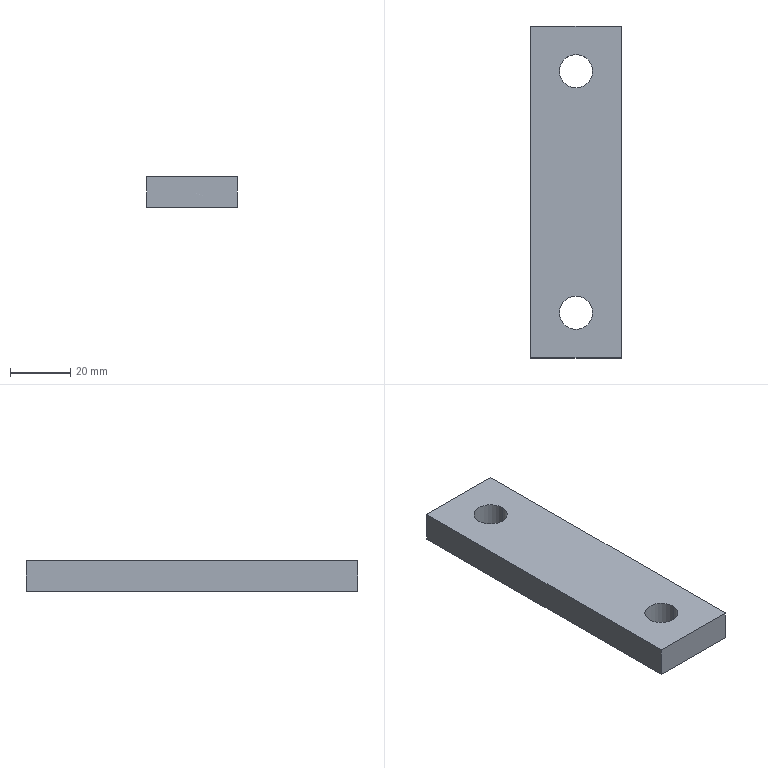Part | STEP file | Adjusting plate clamp | 1 solid | 10 faces | box 30 x 110 x 10 mm | volume 31099 mm3 | plane 6 | cylinder 4 | commonest cylinder face diameters 11 x4
STEP:
#1=CARTESIAN_POINT('',(0.,0.,0.));
#2=DIRECTION('',(0.,0.,1.));
#3=DIRECTION('',(1.,0.,0.));
#4=AXIS2_PLACEMENT_3D('',#1,#2,#3);
#5=CARTESIAN_POINT('',(5.5,-40.,-10.));
#6=VERTEX_POINT('',#5);
#7=CARTESIAN_POINT('',(5.5,-40.,0.));
#8=VERTEX_POINT('',#7);
#9=CARTESIAN_POINT('',(5.5,-40.,-10.));
#10=DIRECTION('',(0.,0.,1.));
#11=VECTOR('',#10,1.);
#12=LINE('',#9,#11);
#13=CARTESIAN_POINT('',(0.,-40.,-10.));
#14=DIRECTION('',(0.,0.,1.));
#15=DIRECTION('',(1.,0.,0.));
#16=AXIS2_PLACEMENT_3D('',#13,#14,#15);
#17=CYLINDRICAL_SURFACE('',#16,5.5);
#18=CARTESIAN_POINT('',(6.283,0.));
#19=DIRECTION('',(0.,1.));
#20=VECTOR('',#19,1.);
#21=LINE('',#18,#20);
#22=(GEOMETRIC_REPRESENTATION_CONTEXT(2)PARAMETRIC_REPRESENTATION_CONTEXT()REPRESENTATION_CONTEXT('',''));
#23=DEFINITIONAL_REPRESENTATION('',(#21),#22);
#24=PCURVE('',#17,#23);
#25=CARTESIAN_POINT('',(0.,-40.,-10.));
#26=DIRECTION('',(0.,0.,1.));
#27=DIRECTION('',(1.,0.,0.));
#28=AXIS2_PLACEMENT_3D('',#25,#26,#27);
#29=CYLINDRICAL_SURFACE('',#28,5.5);
#30=CARTESIAN_POINT('',(0.,0.));
#31=DIRECTION('',(0.,1.));
#32=VECTOR('',#31,1.);
#33=LINE('',#30,#32);
#34=(GEOMETRIC_REPRESENTATION_CONTEXT(2)PARAMETRIC_REPRESENTATION_CONTEXT()REPRESENTATION_CONTEXT('',''));
#35=DEFINITIONAL_REPRESENTATION('',(#33),#34);
#36=PCURVE('',#29,#35);
#37=SURFACE_CURVE('',#12,(#24,#36),.PCURVE_S1.);
#38=EDGE_CURVE('',#6,#8,#37,.T.);
#39=ORIENTED_EDGE('',*,*,#38,.T.);
#40=CARTESIAN_POINT('',(-5.5,-40.,0.));
#41=VERTEX_POINT('',#40);
#42=CARTESIAN_POINT('',(0.,-40.,0.));
#43=DIRECTION('',(0.,0.,1.));
#44=DIRECTION('',(1.,0.,0.));
#45=AXIS2_PLACEMENT_3D('',#42,#43,#44);
#46=CIRCLE('',#45,5.5);
#47=CARTESIAN_POINT('',(0.,10.));
#48=DIRECTION('',(1.,0.));
#49=VECTOR('',#48,1.);
#50=LINE('',#47,#49);
#51=(GEOMETRIC_REPRESENTATION_CONTEXT(2)PARAMETRIC_REPRESENTATION_CONTEXT()REPRESENTATION_CONTEXT('',''));
#52=DEFINITIONAL_REPRESENTATION('',(#50),#51);
#53=PCURVE('',#17,#52);
#54=CARTESIAN_POINT('',(0.,0.,0.));
#55=DIRECTION('',(0.,0.,1.));
#56=DIRECTION('',(1.,0.,0.));
#57=AXIS2_PLACEMENT_3D('',#54,#55,#56);
#58=PLANE('',#57);
#59=CARTESIAN_POINT('',(0.,-40.));
#60=DIRECTION('',(1.,0.));
#61=AXIS2_PLACEMENT_2D('',#59,#60);
#62=CIRCLE('',#61,5.5);
#63=(GEOMETRIC_REPRESENTATION_CONTEXT(2)PARAMETRIC_REPRESENTATION_CONTEXT()REPRESENTATION_CONTEXT('',''));
#64=DEFINITIONAL_REPRESENTATION('',(#62),#63);
#65=PCURVE('',#58,#64);
#66=SURFACE_CURVE('',#46,(#53,#65),.PCURVE_S1.);
#67=EDGE_CURVE('',#41,#8,#66,.T.);
#68=ORIENTED_EDGE('',*,*,#67,.F.);
#69=CARTESIAN_POINT('',(-5.5,-40.,-10.));
#70=VERTEX_POINT('',#69);
#71=CARTESIAN_POINT('',(-5.5,-40.,-10.));
#72=DIRECTION('',(0.,0.,1.));
#73=VECTOR('',#72,1.);
#74=LINE('',#71,#73);
#75=CARTESIAN_POINT('',(3.142,0.));
#76=DIRECTION('',(0.,1.));
#77=VECTOR('',#76,1.);
#78=LINE('',#75,#77);
#79=(GEOMETRIC_REPRESENTATION_CONTEXT(2)PARAMETRIC_REPRESENTATION_CONTEXT()REPRESENTATION_CONTEXT('',''));
#80=DEFINITIONAL_REPRESENTATION('',(#78),#79);
#81=PCURVE('',#17,#80);
#82=CARTESIAN_POINT('',(3.142,0.));
#83=DIRECTION('',(0.,1.));
#84=VECTOR('',#83,1.);
#85=LINE('',#82,#84);
#86=(GEOMETRIC_REPRESENTATION_CONTEXT(2)PARAMETRIC_REPRESENTATION_CONTEXT()REPRESENTATION_CONTEXT('',''));
#87=DEFINITIONAL_REPRESENTATION('',(#85),#86);
#88=PCURVE('',#29,#87);
#89=SURFACE_CURVE('',#74,(#81,#88),.PCURVE_S1.);
#90=EDGE_CURVE('',#70,#41,#89,.T.);
#91=ORIENTED_EDGE('',*,*,#90,.F.);
#92=CARTESIAN_POINT('',(0.,-40.,-10.));
#93=DIRECTION('',(0.,0.,1.));
#94=DIRECTION('',(1.,0.,0.));
#95=AXIS2_PLACEMENT_3D('',#92,#93,#94);
#96=CIRCLE('',#95,5.5);
#97=CARTESIAN_POINT('',(0.,0.));
#98=DIRECTION('',(1.,0.));
#99=VECTOR('',#98,1.);
#100=LINE('',#97,#99);
#101=(GEOMETRIC_REPRESENTATION_CONTEXT(2)PARAMETRIC_REPRESENTATION_CONTEXT()REPRESENTATION_CONTEXT('',''));
#102=DEFINITIONAL_REPRESENTATION('',(#100),#101);
#103=PCURVE('',#17,#102);
#104=CARTESIAN_POINT('',(0.,0.,-10.));
#105=DIRECTION('',(0.,0.,1.));
#106=DIRECTION('',(1.,0.,0.));
#107=AXIS2_PLACEMENT_3D('',#104,#105,#106);
#108=PLANE('',#107);
#109=CARTESIAN_POINT('',(0.,-40.));
#110=DIRECTION('',(1.,0.));
#111=AXIS2_PLACEMENT_2D('',#109,#110);
#112=CIRCLE('',#111,5.5);
#113=(GEOMETRIC_REPRESENTATION_CONTEXT(2)PARAMETRIC_REPRESENTATION_CONTEXT()REPRESENTATION_CONTEXT('',''));
#114=DEFINITIONAL_REPRESENTATION('',(#112),#113);
#115=PCURVE('',#108,#114);
#116=SURFACE_CURVE('',#96,(#103,#115),.PCURVE_S1.);
#117=EDGE_CURVE('',#70,#6,#116,.T.);
#118=ORIENTED_EDGE('',*,*,#117,.T.);
#119=EDGE_LOOP('',(#39,#68,#91,#118));
#120=FACE_BOUND('',#119,.F.);
#121=ADVANCED_FACE('',(#120),#17,.F.);
#122=CARTESIAN_POINT('',(5.5,40.,-10.));
#123=VERTEX_POINT('',#122);
#124=CARTESIAN_POINT('',(5.5,40.,0.));
#125=VERTEX_POINT('',#124);
#126=CARTESIAN_POINT('',(5.5,40.,-10.));
#127=DIRECTION('',(0.,0.,1.));
#128=VECTOR('',#127,1.);
#129=LINE('',#126,#128);
#130=CARTESIAN_POINT('',(0.,40.,-10.));
#131=DIRECTION('',(0.,0.,1.));
#132=DIRECTION('',(1.,0.,0.));
#133=AXIS2_PLACEMENT_3D('',#130,#131,#132);
#134=CYLINDRICAL_SURFACE('',#133,5.5);
#135=CARTESIAN_POINT('',(6.283,0.));
#136=DIRECTION('',(0.,1.));
#137=VECTOR('',#136,1.);
#138=LINE('',#135,#137);
#139=(GEOMETRIC_REPRESENTATION_CONTEXT(2)PARAMETRIC_REPRESENTATION_CONTEXT()REPRESENTATION_CONTEXT('',''));
#140=DEFINITIONAL_REPRESENTATION('',(#138),#139);
#141=PCURVE('',#134,#140);
#142=CARTESIAN_POINT('',(0.,40.,-10.));
#143=DIRECTION('',(0.,0.,1.));
#144=DIRECTION('',(1.,0.,0.));
#145=AXIS2_PLACEMENT_3D('',#142,#143,#144);
#146=CYLINDRICAL_SURFACE('',#145,5.5);
#147=CARTESIAN_POINT('',(0.,0.));
#148=DIRECTION('',(0.,1.));
#149=VECTOR('',#148,1.);
#150=LINE('',#147,#149);
#151=(GEOMETRIC_REPRESENTATION_CONTEXT(2)PARAMETRIC_REPRESENTATION_CONTEXT()REPRESENTATION_CONTEXT('',''));
#152=DEFINITIONAL_REPRESENTATION('',(#150),#151);
#153=PCURVE('',#146,#152);
#154=SURFACE_CURVE('',#129,(#141,#153),.PCURVE_S1.);
#155=EDGE_CURVE('',#123,#125,#154,.T.);
#156=ORIENTED_EDGE('',*,*,#155,.T.);
#157=CARTESIAN_POINT('',(-5.5,40.,0.));
#158=VERTEX_POINT('',#157);
#159=CARTESIAN_POINT('',(0.,40.,0.));
#160=DIRECTION('',(0.,0.,1.));
#161=DIRECTION('',(1.,0.,0.));
#162=AXIS2_PLACEMENT_3D('',#159,#160,#161);
#163=CIRCLE('',#162,5.5);
#164=CARTESIAN_POINT('',(0.,10.));
#165=DIRECTION('',(1.,0.));
#166=VECTOR('',#165,1.);
#167=LINE('',#164,#166);
#168=(GEOMETRIC_REPRESENTATION_CONTEXT(2)PARAMETRIC_REPRESENTATION_CONTEXT()REPRESENTATION_CONTEXT('',''));
#169=DEFINITIONAL_REPRESENTATION('',(#167),#168);
#170=PCURVE('',#134,#169);
#171=CARTESIAN_POINT('',(0.,40.));
#172=DIRECTION('',(1.,0.));
#173=AXIS2_PLACEMENT_2D('',#171,#172);
#174=CIRCLE('',#173,5.5);
#175=(GEOMETRIC_REPRESENTATION_CONTEXT(2)PARAMETRIC_REPRESENTATION_CONTEXT()REPRESENTATION_CONTEXT('',''));
#176=DEFINITIONAL_REPRESENTATION('',(#174),#175);
#177=PCURVE('',#58,#176);
#178=SURFACE_CURVE('',#163,(#170,#177),.PCURVE_S1.);
#179=EDGE_CURVE('',#158,#125,#178,.T.);
#180=ORIENTED_EDGE('',*,*,#179,.F.);
#181=CARTESIAN_POINT('',(-5.5,40.,-10.));
#182=VERTEX_POINT('',#181);
#183=CARTESIAN_POINT('',(-5.5,40.,-10.));
#184=DIRECTION('',(0.,0.,1.));
#185=VECTOR('',#184,1.);
#186=LINE('',#183,#185);
#187=CARTESIAN_POINT('',(3.142,0.));
#188=DIRECTION('',(0.,1.));
#189=VECTOR('',#188,1.);
#190=LINE('',#187,#189);
#191=(GEOMETRIC_REPRESENTATION_CONTEXT(2)PARAMETRIC_REPRESENTATION_CONTEXT()REPRESENTATION_CONTEXT('',''));
#192=DEFINITIONAL_REPRESENTATION('',(#190),#191);
#193=PCURVE('',#134,#192);
#194=CARTESIAN_POINT('',(3.142,0.));
#195=DIRECTION('',(0.,1.));
#196=VECTOR('',#195,1.);
#197=LINE('',#194,#196);
#198=(GEOMETRIC_REPRESENTATION_CONTEXT(2)PARAMETRIC_REPRESENTATION_CONTEXT()REPRESENTATION_CONTEXT('',''));
#199=DEFINITIONAL_REPRESENTATION('',(#197),#198);
#200=PCURVE('',#146,#199);
#201=SURFACE_CURVE('',#186,(#193,#200),.PCURVE_S1.);
#202=EDGE_CURVE('',#182,#158,#201,.T.);
#203=ORIENTED_EDGE('',*,*,#202,.F.);
#204=CARTESIAN_POINT('',(0.,40.,-10.));
#205=DIRECTION('',(0.,0.,1.));
#206=DIRECTION('',(1.,0.,0.));
#207=AXIS2_PLACEMENT_3D('',#204,#205,#206);
#208=CIRCLE('',#207,5.5);
#209=CARTESIAN_POINT('',(0.,0.));
#210=DIRECTION('',(1.,0.));
#211=VECTOR('',#210,1.);
#212=LINE('',#209,#211);
#213=(GEOMETRIC_REPRESENTATION_CONTEXT(2)PARAMETRIC_REPRESENTATION_CONTEXT()REPRESENTATION_CONTEXT('',''));
#214=DEFINITIONAL_REPRESENTATION('',(#212),#213);
#215=PCURVE('',#134,#214);
#216=CARTESIAN_POINT('',(0.,40.));
#217=DIRECTION('',(1.,0.));
#218=AXIS2_PLACEMENT_2D('',#216,#217);
#219=CIRCLE('',#218,5.5);
#220=(GEOMETRIC_REPRESENTATION_CONTEXT(2)PARAMETRIC_REPRESENTATION_CONTEXT()REPRESENTATION_CONTEXT('',''));
#221=DEFINITIONAL_REPRESENTATION('',(#219),#220);
#222=PCURVE('',#108,#221);
#223=SURFACE_CURVE('',#208,(#215,#222),.PCURVE_S1.);
#224=EDGE_CURVE('',#182,#123,#223,.T.);
#225=ORIENTED_EDGE('',*,*,#224,.T.);
#226=EDGE_LOOP('',(#156,#180,#203,#225));
#227=FACE_BOUND('',#226,.F.);
#228=ADVANCED_FACE('',(#227),#134,.F.);
#229=CARTESIAN_POINT('',(-15.,55.,0.));
#230=VERTEX_POINT('',#229);
#231=CARTESIAN_POINT('',(-15.,-55.,0.));
#232=VERTEX_POINT('',#231);
#233=CARTESIAN_POINT('',(-15.,55.,0.));
#234=DIRECTION('',(0.,-1.,0.));
#235=VECTOR('',#234,1.);
#236=LINE('',#233,#235);
#237=CARTESIAN_POINT('',(-15.,55.,-10.));
#238=DIRECTION('',(-1.,0.,0.));
#239=DIRECTION('',(0.,0.,1.));
#240=AXIS2_PLACEMENT_3D('',#237,#238,#239);
#241=PLANE('',#240);
#242=CARTESIAN_POINT('',(10.,0.));
#243=DIRECTION('',(0.,-1.));
#244=VECTOR('',#243,1.);
#245=LINE('',#242,#244);
#246=(GEOMETRIC_REPRESENTATION_CONTEXT(2)PARAMETRIC_REPRESENTATION_CONTEXT()REPRESENTATION_CONTEXT('',''));
#247=DEFINITIONAL_REPRESENTATION('',(#245),#246);
#248=PCURVE('',#241,#247);
#249=CARTESIAN_POINT('',(-15.,55.));
#250=DIRECTION('',(0.,-1.));
#251=VECTOR('',#250,1.);
#252=LINE('',#249,#251);
#253=(GEOMETRIC_REPRESENTATION_CONTEXT(2)PARAMETRIC_REPRESENTATION_CONTEXT()REPRESENTATION_CONTEXT('',''));
#254=DEFINITIONAL_REPRESENTATION('',(#252),#253);
#255=PCURVE('',#58,#254);
#256=SURFACE_CURVE('',#236,(#248,#255),.PCURVE_S1.);
#257=EDGE_CURVE('',#230,#232,#256,.T.);
#258=ORIENTED_EDGE('',*,*,#257,.F.);
#259=CARTESIAN_POINT('',(-15.,55.,-10.));
#260=VERTEX_POINT('',#259);
#261=CARTESIAN_POINT('',(-15.,55.,-10.));
#262=DIRECTION('',(0.,0.,1.));
#263=VECTOR('',#262,1.);
#264=LINE('',#261,#263);
#265=CARTESIAN_POINT('',(0.,0.));
#266=DIRECTION('',(1.,0.));
#267=VECTOR('',#266,1.);
#268=LINE('',#265,#267);
#269=(GEOMETRIC_REPRESENTATION_CONTEXT(2)PARAMETRIC_REPRESENTATION_CONTEXT()REPRESENTATION_CONTEXT('',''));
#270=DEFINITIONAL_REPRESENTATION('',(#268),#269);
#271=PCURVE('',#241,#270);
#272=CARTESIAN_POINT('',(-15.,55.,-10.));
#273=DIRECTION('',(0.,1.,0.));
#274=DIRECTION('',(0.,0.,1.));
#275=AXIS2_PLACEMENT_3D('',#272,#273,#274);
#276=PLANE('',#275);
#277=CARTESIAN_POINT('',(0.,0.));
#278=DIRECTION('',(1.,0.));
#279=VECTOR('',#278,1.);
#280=LINE('',#277,#279);
#281=(GEOMETRIC_REPRESENTATION_CONTEXT(2)PARAMETRIC_REPRESENTATION_CONTEXT()REPRESENTATION_CONTEXT('',''));
#282=DEFINITIONAL_REPRESENTATION('',(#280),#281);
#283=PCURVE('',#276,#282);
#284=SURFACE_CURVE('',#264,(#271,#283),.PCURVE_S1.);
#285=EDGE_CURVE('',#260,#230,#284,.T.);
#286=ORIENTED_EDGE('',*,*,#285,.F.);
#287=CARTESIAN_POINT('',(-15.,-55.,-10.));
#288=VERTEX_POINT('',#287);
#289=CARTESIAN_POINT('',(-15.,55.,-10.));
#290=DIRECTION('',(0.,-1.,0.));
#291=VECTOR('',#290,1.);
#292=LINE('',#289,#291);
#293=CARTESIAN_POINT('',(0.,0.));
#294=DIRECTION('',(0.,-1.));
#295=VECTOR('',#294,1.);
#296=LINE('',#293,#295);
#297=(GEOMETRIC_REPRESENTATION_CONTEXT(2)PARAMETRIC_REPRESENTATION_CONTEXT()REPRESENTATION_CONTEXT('',''));
#298=DEFINITIONAL_REPRESENTATION('',(#296),#297);
#299=PCURVE('',#241,#298);
#300=CARTESIAN_POINT('',(-15.,55.));
#301=DIRECTION('',(0.,-1.));
#302=VECTOR('',#301,1.);
#303=LINE('',#300,#302);
#304=(GEOMETRIC_REPRESENTATION_CONTEXT(2)PARAMETRIC_REPRESENTATION_CONTEXT()REPRESENTATION_CONTEXT('',''));
#305=DEFINITIONAL_REPRESENTATION('',(#303),#304);
#306=PCURVE('',#108,#305);
#307=SURFACE_CURVE('',#292,(#299,#306),.PCURVE_S1.);
#308=EDGE_CURVE('',#260,#288,#307,.T.);
#309=ORIENTED_EDGE('',*,*,#308,.T.);
#310=CARTESIAN_POINT('',(-15.,-55.,-10.));
#311=DIRECTION('',(0.,0.,1.));
#312=VECTOR('',#311,1.);
#313=LINE('',#310,#312);
#314=CARTESIAN_POINT('',(0.,-110.));
#315=DIRECTION('',(1.,0.));
#316=VECTOR('',#315,1.);
#317=LINE('',#314,#316);
#318=(GEOMETRIC_REPRESENTATION_CONTEXT(2)PARAMETRIC_REPRESENTATION_CONTEXT()REPRESENTATION_CONTEXT('',''));
#319=DEFINITIONAL_REPRESENTATION('',(#317),#318);
#320=PCURVE('',#241,#319);
#321=CARTESIAN_POINT('',(-15.,-55.,-10.));
#322=DIRECTION('',(0.,-1.,0.));
#323=DIRECTION('',(0.,0.,-1.));
#324=AXIS2_PLACEMENT_3D('',#321,#322,#323);
#325=PLANE('',#324);
#326=CARTESIAN_POINT('',(0.,0.));
#327=DIRECTION('',(-1.,0.));
#328=VECTOR('',#327,1.);
#329=LINE('',#326,#328);
#330=(GEOMETRIC_REPRESENTATION_CONTEXT(2)PARAMETRIC_REPRESENTATION_CONTEXT()REPRESENTATION_CONTEXT('',''));
#331=DEFINITIONAL_REPRESENTATION('',(#329),#330);
#332=PCURVE('',#325,#331);
#333=SURFACE_CURVE('',#313,(#320,#332),.PCURVE_S1.);
#334=EDGE_CURVE('',#288,#232,#333,.T.);
#335=ORIENTED_EDGE('',*,*,#334,.T.);
#336=EDGE_LOOP('',(#258,#286,#309,#335));
#337=FACE_BOUND('',#336,.T.);
#338=ADVANCED_FACE('',(#337),#241,.T.);
#339=CARTESIAN_POINT('',(15.,55.,0.));
#340=VERTEX_POINT('',#339);
#341=CARTESIAN_POINT('',(-15.,55.,0.));
#342=DIRECTION('',(-1.,0.,0.));
#343=VECTOR('',#342,1.);
#344=LINE('',#341,#343);
#345=CARTESIAN_POINT('',(10.,0.));
#346=DIRECTION('',(0.,-1.));
#347=VECTOR('',#346,1.);
#348=LINE('',#345,#347);
#349=(GEOMETRIC_REPRESENTATION_CONTEXT(2)PARAMETRIC_REPRESENTATION_CONTEXT()REPRESENTATION_CONTEXT('',''));
#350=DEFINITIONAL_REPRESENTATION('',(#348),#349);
#351=PCURVE('',#276,#350);
#352=CARTESIAN_POINT('',(-15.,55.));
#353=DIRECTION('',(-1.,0.));
#354=VECTOR('',#353,1.);
#355=LINE('',#352,#354);
#356=(GEOMETRIC_REPRESENTATION_CONTEXT(2)PARAMETRIC_REPRESENTATION_CONTEXT()REPRESENTATION_CONTEXT('',''));
#357=DEFINITIONAL_REPRESENTATION('',(#355),#356);
#358=PCURVE('',#58,#357);
#359=SURFACE_CURVE('',#344,(#351,#358),.PCURVE_S1.);
#360=EDGE_CURVE('',#340,#230,#359,.T.);
#361=ORIENTED_EDGE('',*,*,#360,.F.);
#362=CARTESIAN_POINT('',(15.,55.,-10.));
#363=VERTEX_POINT('',#362);
#364=CARTESIAN_POINT('',(15.,55.,-10.));
#365=DIRECTION('',(0.,0.,1.));
#366=VECTOR('',#365,1.);
#367=LINE('',#364,#366);
#368=CARTESIAN_POINT('',(0.,30.));
#369=DIRECTION('',(1.,0.));
#370=VECTOR('',#369,1.);
#371=LINE('',#368,#370);
#372=(GEOMETRIC_REPRESENTATION_CONTEXT(2)PARAMETRIC_REPRESENTATION_CONTEXT()REPRESENTATION_CONTEXT('',''));
#373=DEFINITIONAL_REPRESENTATION('',(#371),#372);
#374=PCURVE('',#276,#373);
#375=CARTESIAN_POINT('',(15.,55.,-10.));
#376=DIRECTION('',(1.,0.,0.));
#377=DIRECTION('',(0.,0.,-1.));
#378=AXIS2_PLACEMENT_3D('',#375,#376,#377);
#379=PLANE('',#378);
#380=CARTESIAN_POINT('',(0.,0.));
#381=DIRECTION('',(-1.,0.));
#382=VECTOR('',#381,1.);
#383=LINE('',#380,#382);
#384=(GEOMETRIC_REPRESENTATION_CONTEXT(2)PARAMETRIC_REPRESENTATION_CONTEXT()REPRESENTATION_CONTEXT('',''));
#385=DEFINITIONAL_REPRESENTATION('',(#383),#384);
#386=PCURVE('',#379,#385);
#387=SURFACE_CURVE('',#367,(#374,#386),.PCURVE_S1.);
#388=EDGE_CURVE('',#363,#340,#387,.T.);
#389=ORIENTED_EDGE('',*,*,#388,.F.);
#390=CARTESIAN_POINT('',(-15.,55.,-10.));
#391=DIRECTION('',(-1.,0.,0.));
#392=VECTOR('',#391,1.);
#393=LINE('',#390,#392);
#394=CARTESIAN_POINT('',(0.,0.));
#395=DIRECTION('',(0.,-1.));
#396=VECTOR('',#395,1.);
#397=LINE('',#394,#396);
#398=(GEOMETRIC_REPRESENTATION_CONTEXT(2)PARAMETRIC_REPRESENTATION_CONTEXT()REPRESENTATION_CONTEXT('',''));
#399=DEFINITIONAL_REPRESENTATION('',(#397),#398);
#400=PCURVE('',#276,#399);
#401=CARTESIAN_POINT('',(-15.,55.));
#402=DIRECTION('',(-1.,0.));
#403=VECTOR('',#402,1.);
#404=LINE('',#401,#403);
#405=(GEOMETRIC_REPRESENTATION_CONTEXT(2)PARAMETRIC_REPRESENTATION_CONTEXT()REPRESENTATION_CONTEXT('',''));
#406=DEFINITIONAL_REPRESENTATION('',(#404),#405);
#407=PCURVE('',#108,#406);
#408=SURFACE_CURVE('',#393,(#400,#407),.PCURVE_S1.);
#409=EDGE_CURVE('',#363,#260,#408,.T.);
#410=ORIENTED_EDGE('',*,*,#409,.T.);
#411=ORIENTED_EDGE('',*,*,#285,.T.);
#412=EDGE_LOOP('',(#361,#389,#410,#411));
#413=FACE_BOUND('',#412,.T.);
#414=ADVANCED_FACE('',(#413),#276,.T.);
#415=CARTESIAN_POINT('',(15.,-55.,0.));
#416=VERTEX_POINT('',#415);
#417=CARTESIAN_POINT('',(15.,55.,0.));
#418=DIRECTION('',(0.,1.,0.));
#419=VECTOR('',#418,1.);
#420=LINE('',#417,#419);
#421=CARTESIAN_POINT('',(-10.,0.));
#422=DIRECTION('',(0.,1.));
#423=VECTOR('',#422,1.);
#424=LINE('',#421,#423);
#425=(GEOMETRIC_REPRESENTATION_CONTEXT(2)PARAMETRIC_REPRESENTATION_CONTEXT()REPRESENTATION_CONTEXT('',''));
#426=DEFINITIONAL_REPRESENTATION('',(#424),#425);
#427=PCURVE('',#379,#426);
#428=CARTESIAN_POINT('',(15.,55.));
#429=DIRECTION('',(0.,1.));
#430=VECTOR('',#429,1.);
#431=LINE('',#428,#430);
#432=(GEOMETRIC_REPRESENTATION_CONTEXT(2)PARAMETRIC_REPRESENTATION_CONTEXT()REPRESENTATION_CONTEXT('',''));
#433=DEFINITIONAL_REPRESENTATION('',(#431),#432);
#434=PCURVE('',#58,#433);
#435=SURFACE_CURVE('',#420,(#427,#434),.PCURVE_S1.);
#436=EDGE_CURVE('',#416,#340,#435,.T.);
#437=ORIENTED_EDGE('',*,*,#436,.F.);
#438=CARTESIAN_POINT('',(15.,-55.,-10.));
#439=VERTEX_POINT('',#438);
#440=CARTESIAN_POINT('',(15.,-55.,-10.));
#441=DIRECTION('',(0.,0.,1.));
#442=VECTOR('',#441,1.);
#443=LINE('',#440,#442);
#444=CARTESIAN_POINT('',(0.,-110.));
#445=DIRECTION('',(-1.,0.));
#446=VECTOR('',#445,1.);
#447=LINE('',#444,#446);
#448=(GEOMETRIC_REPRESENTATION_CONTEXT(2)PARAMETRIC_REPRESENTATION_CONTEXT()REPRESENTATION_CONTEXT('',''));
#449=DEFINITIONAL_REPRESENTATION('',(#447),#448);
#450=PCURVE('',#379,#449);
#451=CARTESIAN_POINT('',(0.,30.));
#452=DIRECTION('',(-1.,0.));
#453=VECTOR('',#452,1.);
#454=LINE('',#451,#453);
#455=(GEOMETRIC_REPRESENTATION_CONTEXT(2)PARAMETRIC_REPRESENTATION_CONTEXT()REPRESENTATION_CONTEXT('',''));
#456=DEFINITIONAL_REPRESENTATION('',(#454),#455);
#457=PCURVE('',#325,#456);
#458=SURFACE_CURVE('',#443,(#450,#457),.PCURVE_S1.);
#459=EDGE_CURVE('',#439,#416,#458,.T.);
#460=ORIENTED_EDGE('',*,*,#459,.F.);
#461=CARTESIAN_POINT('',(15.,55.,-10.));
#462=DIRECTION('',(0.,1.,0.));
#463=VECTOR('',#462,1.);
#464=LINE('',#461,#463);
#465=CARTESIAN_POINT('',(0.,0.));
#466=DIRECTION('',(0.,1.));
#467=VECTOR('',#466,1.);
#468=LINE('',#465,#467);
#469=(GEOMETRIC_REPRESENTATION_CONTEXT(2)PARAMETRIC_REPRESENTATION_CONTEXT()REPRESENTATION_CONTEXT('',''));
#470=DEFINITIONAL_REPRESENTATION('',(#468),#469);
#471=PCURVE('',#379,#470);
#472=CARTESIAN_POINT('',(15.,55.));
#473=DIRECTION('',(0.,1.));
#474=VECTOR('',#473,1.);
#475=LINE('',#472,#474);
#476=(GEOMETRIC_REPRESENTATION_CONTEXT(2)PARAMETRIC_REPRESENTATION_CONTEXT()REPRESENTATION_CONTEXT('',''));
#477=DEFINITIONAL_REPRESENTATION('',(#475),#476);
#478=PCURVE('',#108,#477);
#479=SURFACE_CURVE('',#464,(#471,#478),.PCURVE_S1.);
#480=EDGE_CURVE('',#439,#363,#479,.T.);
#481=ORIENTED_EDGE('',*,*,#480,.T.);
#482=ORIENTED_EDGE('',*,*,#388,.T.);
#483=EDGE_LOOP('',(#437,#460,#481,#482));
#484=FACE_BOUND('',#483,.T.);
#485=ADVANCED_FACE('',(#484),#379,.T.);
#486=CARTESIAN_POINT('',(-15.,-55.,0.));
#487=DIRECTION('',(1.,0.,0.));
#488=VECTOR('',#487,1.);
#489=LINE('',#486,#488);
#490=CARTESIAN_POINT('',(-10.,0.));
#491=DIRECTION('',(0.,1.));
#492=VECTOR('',#491,1.);
#493=LINE('',#490,#492);
#494=(GEOMETRIC_REPRESENTATION_CONTEXT(2)PARAMETRIC_REPRESENTATION_CONTEXT()REPRESENTATION_CONTEXT('',''));
#495=DEFINITIONAL_REPRESENTATION('',(#493),#494);
#496=PCURVE('',#325,#495);
#497=CARTESIAN_POINT('',(-15.,-55.));
#498=DIRECTION('',(1.,0.));
#499=VECTOR('',#498,1.);
#500=LINE('',#497,#499);
#501=(GEOMETRIC_REPRESENTATION_CONTEXT(2)PARAMETRIC_REPRESENTATION_CONTEXT()REPRESENTATION_CONTEXT('',''));
#502=DEFINITIONAL_REPRESENTATION('',(#500),#501);
#503=PCURVE('',#58,#502);
#504=SURFACE_CURVE('',#489,(#496,#503),.PCURVE_S1.);
#505=EDGE_CURVE('',#232,#416,#504,.T.);
#506=ORIENTED_EDGE('',*,*,#505,.F.);
#507=ORIENTED_EDGE('',*,*,#334,.F.);
#508=CARTESIAN_POINT('',(-15.,-55.,-10.));
#509=DIRECTION('',(1.,0.,0.));
#510=VECTOR('',#509,1.);
#511=LINE('',#508,#510);
#512=CARTESIAN_POINT('',(0.,0.));
#513=DIRECTION('',(0.,1.));
#514=VECTOR('',#513,1.);
#515=LINE('',#512,#514);
#516=(GEOMETRIC_REPRESENTATION_CONTEXT(2)PARAMETRIC_REPRESENTATION_CONTEXT()REPRESENTATION_CONTEXT('',''));
#517=DEFINITIONAL_REPRESENTATION('',(#515),#516);
#518=PCURVE('',#325,#517);
#519=CARTESIAN_POINT('',(-15.,-55.));
#520=DIRECTION('',(1.,0.));
#521=VECTOR('',#520,1.);
#522=LINE('',#519,#521);
#523=(GEOMETRIC_REPRESENTATION_CONTEXT(2)PARAMETRIC_REPRESENTATION_CONTEXT()REPRESENTATION_CONTEXT('',''));
#524=DEFINITIONAL_REPRESENTATION('',(#522),#523);
#525=PCURVE('',#108,#524);
#526=SURFACE_CURVE('',#511,(#518,#525),.PCURVE_S1.);
#527=EDGE_CURVE('',#288,#439,#526,.T.);
#528=ORIENTED_EDGE('',*,*,#527,.T.);
#529=ORIENTED_EDGE('',*,*,#459,.T.);
#530=EDGE_LOOP('',(#506,#507,#528,#529));
#531=FACE_BOUND('',#530,.T.);
#532=ADVANCED_FACE('',(#531),#325,.T.);
#533=CARTESIAN_POINT('',(0.,-40.,-10.));
#534=DIRECTION('',(0.,0.,1.));
#535=DIRECTION('',(1.,0.,0.));
#536=AXIS2_PLACEMENT_3D('',#533,#534,#535);
#537=CIRCLE('',#536,5.5);
#538=CARTESIAN_POINT('',(0.,-40.));
#539=DIRECTION('',(1.,0.));
#540=AXIS2_PLACEMENT_2D('',#538,#539);
#541=CIRCLE('',#540,5.5);
#542=(GEOMETRIC_REPRESENTATION_CONTEXT(2)PARAMETRIC_REPRESENTATION_CONTEXT()REPRESENTATION_CONTEXT('',''));
#543=DEFINITIONAL_REPRESENTATION('',(#541),#542);
#544=PCURVE('',#108,#543);
#545=CARTESIAN_POINT('',(0.,0.));
#546=DIRECTION('',(1.,0.));
#547=VECTOR('',#546,1.);
#548=LINE('',#545,#547);
#549=(GEOMETRIC_REPRESENTATION_CONTEXT(2)PARAMETRIC_REPRESENTATION_CONTEXT()REPRESENTATION_CONTEXT('',''));
#550=DEFINITIONAL_REPRESENTATION('',(#548),#549);
#551=PCURVE('',#29,#550);
#552=SURFACE_CURVE('',#537,(#544,#551),.PCURVE_S1.);
#553=EDGE_CURVE('',#6,#70,#552,.T.);
#554=ORIENTED_EDGE('',*,*,#553,.T.);
#555=ORIENTED_EDGE('',*,*,#117,.T.);
#556=EDGE_LOOP('',(#554,#555));
#557=FACE_BOUND('',#556,.T.);
#558=CARTESIAN_POINT('',(0.,40.,-10.));
#559=DIRECTION('',(0.,0.,1.));
#560=DIRECTION('',(1.,0.,0.));
#561=AXIS2_PLACEMENT_3D('',#558,#559,#560);
#562=CIRCLE('',#561,5.5);
#563=CARTESIAN_POINT('',(0.,40.));
#564=DIRECTION('',(1.,0.));
#565=AXIS2_PLACEMENT_2D('',#563,#564);
#566=CIRCLE('',#565,5.5);
#567=(GEOMETRIC_REPRESENTATION_CONTEXT(2)PARAMETRIC_REPRESENTATION_CONTEXT()REPRESENTATION_CONTEXT('',''));
#568=DEFINITIONAL_REPRESENTATION('',(#566),#567);
#569=PCURVE('',#108,#568);
#570=CARTESIAN_POINT('',(0.,0.));
#571=DIRECTION('',(1.,0.));
#572=VECTOR('',#571,1.);
#573=LINE('',#570,#572);
#574=(GEOMETRIC_REPRESENTATION_CONTEXT(2)PARAMETRIC_REPRESENTATION_CONTEXT()REPRESENTATION_CONTEXT('',''));
#575=DEFINITIONAL_REPRESENTATION('',(#573),#574);
#576=PCURVE('',#146,#575);
#577=SURFACE_CURVE('',#562,(#569,#576),.PCURVE_S1.);
#578=EDGE_CURVE('',#123,#182,#577,.T.);
#579=ORIENTED_EDGE('',*,*,#578,.T.);
#580=ORIENTED_EDGE('',*,*,#224,.T.);
#581=EDGE_LOOP('',(#579,#580));
#582=FACE_BOUND('',#581,.T.);
#583=ORIENTED_EDGE('',*,*,#308,.F.);
#584=ORIENTED_EDGE('',*,*,#409,.F.);
#585=ORIENTED_EDGE('',*,*,#480,.F.);
#586=ORIENTED_EDGE('',*,*,#527,.F.);
#587=EDGE_LOOP('',(#583,#584,#585,#586));
#588=FACE_BOUND('',#587,.T.);
#589=ADVANCED_FACE('',(#557,#582,#588),#108,.F.);
#590=CARTESIAN_POINT('',(0.,-40.,0.));
#591=DIRECTION('',(0.,0.,1.));
#592=DIRECTION('',(1.,0.,0.));
#593=AXIS2_PLACEMENT_3D('',#590,#591,#592);
#594=CIRCLE('',#593,5.5);
#595=CARTESIAN_POINT('',(0.,-40.));
#596=DIRECTION('',(1.,0.));
#597=AXIS2_PLACEMENT_2D('',#595,#596);
#598=CIRCLE('',#597,5.5);
#599=(GEOMETRIC_REPRESENTATION_CONTEXT(2)PARAMETRIC_REPRESENTATION_CONTEXT()REPRESENTATION_CONTEXT('',''));
#600=DEFINITIONAL_REPRESENTATION('',(#598),#599);
#601=PCURVE('',#58,#600);
#602=CARTESIAN_POINT('',(0.,10.));
#603=DIRECTION('',(1.,0.));
#604=VECTOR('',#603,1.);
#605=LINE('',#602,#604);
#606=(GEOMETRIC_REPRESENTATION_CONTEXT(2)PARAMETRIC_REPRESENTATION_CONTEXT()REPRESENTATION_CONTEXT('',''));
#607=DEFINITIONAL_REPRESENTATION('',(#605),#606);
#608=PCURVE('',#29,#607);
#609=SURFACE_CURVE('',#594,(#601,#608),.PCURVE_S1.);
#610=EDGE_CURVE('',#8,#41,#609,.T.);
#611=ORIENTED_EDGE('',*,*,#610,.F.);
#612=ORIENTED_EDGE('',*,*,#67,.F.);
#613=EDGE_LOOP('',(#611,#612));
#614=FACE_BOUND('',#613,.T.);
#615=CARTESIAN_POINT('',(0.,40.,0.));
#616=DIRECTION('',(0.,0.,1.));
#617=DIRECTION('',(1.,0.,0.));
#618=AXIS2_PLACEMENT_3D('',#615,#616,#617);
#619=CIRCLE('',#618,5.5);
#620=CARTESIAN_POINT('',(0.,40.));
#621=DIRECTION('',(1.,0.));
#622=AXIS2_PLACEMENT_2D('',#620,#621);
#623=CIRCLE('',#622,5.5);
#624=(GEOMETRIC_REPRESENTATION_CONTEXT(2)PARAMETRIC_REPRESENTATION_CONTEXT()REPRESENTATION_CONTEXT('',''));
#625=DEFINITIONAL_REPRESENTATION('',(#623),#624);
#626=PCURVE('',#58,#625);
#627=CARTESIAN_POINT('',(0.,10.));
#628=DIRECTION('',(1.,0.));
#629=VECTOR('',#628,1.);
#630=LINE('',#627,#629);
#631=(GEOMETRIC_REPRESENTATION_CONTEXT(2)PARAMETRIC_REPRESENTATION_CONTEXT()REPRESENTATION_CONTEXT('',''));
#632=DEFINITIONAL_REPRESENTATION('',(#630),#631);
#633=PCURVE('',#146,#632);
#634=SURFACE_CURVE('',#619,(#626,#633),.PCURVE_S1.);
#635=EDGE_CURVE('',#125,#158,#634,.T.);
#636=ORIENTED_EDGE('',*,*,#635,.F.);
#637=ORIENTED_EDGE('',*,*,#179,.F.);
#638=EDGE_LOOP('',(#636,#637));
#639=FACE_BOUND('',#638,.T.);
#640=ORIENTED_EDGE('',*,*,#257,.T.);
#641=ORIENTED_EDGE('',*,*,#505,.T.);
#642=ORIENTED_EDGE('',*,*,#436,.T.);
#643=ORIENTED_EDGE('',*,*,#360,.T.);
#644=EDGE_LOOP('',(#640,#641,#642,#643));
#645=FACE_BOUND('',#644,.T.);
#646=ADVANCED_FACE('',(#614,#639,#645),#58,.T.);
#647=ORIENTED_EDGE('',*,*,#635,.F.);
#648=ORIENTED_EDGE('',*,*,#155,.F.);
#649=ORIENTED_EDGE('',*,*,#578,.T.);
#650=ORIENTED_EDGE('',*,*,#202,.T.);
#651=EDGE_LOOP('',(#647,#648,#649,#650));
#652=FACE_BOUND('',#651,.F.);
#653=ADVANCED_FACE('',(#652),#146,.F.);
#654=ORIENTED_EDGE('',*,*,#610,.F.);
#655=ORIENTED_EDGE('',*,*,#38,.F.);
#656=ORIENTED_EDGE('',*,*,#553,.T.);
#657=ORIENTED_EDGE('',*,*,#90,.T.);
#658=EDGE_LOOP('',(#654,#655,#656,#657));
#659=FACE_BOUND('',#658,.F.);
#660=ADVANCED_FACE('',(#659),#29,.F.);
#661=CLOSED_SHELL('',(#121,#228,#338,#414,#485,#532,#589,#646,#653,#660));
#662=MANIFOLD_SOLID_BREP('',#661);
#663=(LENGTH_UNIT()NAMED_UNIT(*)SI_UNIT(.MILLI.,.METRE.));
#664=UNCERTAINTY_MEASURE_WITH_UNIT(LENGTH_MEASURE(0.0000001),#663,'','');
#665=(NAMED_UNIT(*)PLANE_ANGLE_UNIT()SI_UNIT($,.RADIAN.));
#666=(NAMED_UNIT(*)SI_UNIT($,.STERADIAN.)SOLID_ANGLE_UNIT());
#667=(GEOMETRIC_REPRESENTATION_CONTEXT(3)GLOBAL_UNCERTAINTY_ASSIGNED_CONTEXT((#664))GLOBAL_UNIT_ASSIGNED_CONTEXT((#663,#665,#666))REPRESENTATION_CONTEXT('',''));
#668=ADVANCED_BREP_SHAPE_REPRESENTATION('',(#4,#662),#667);